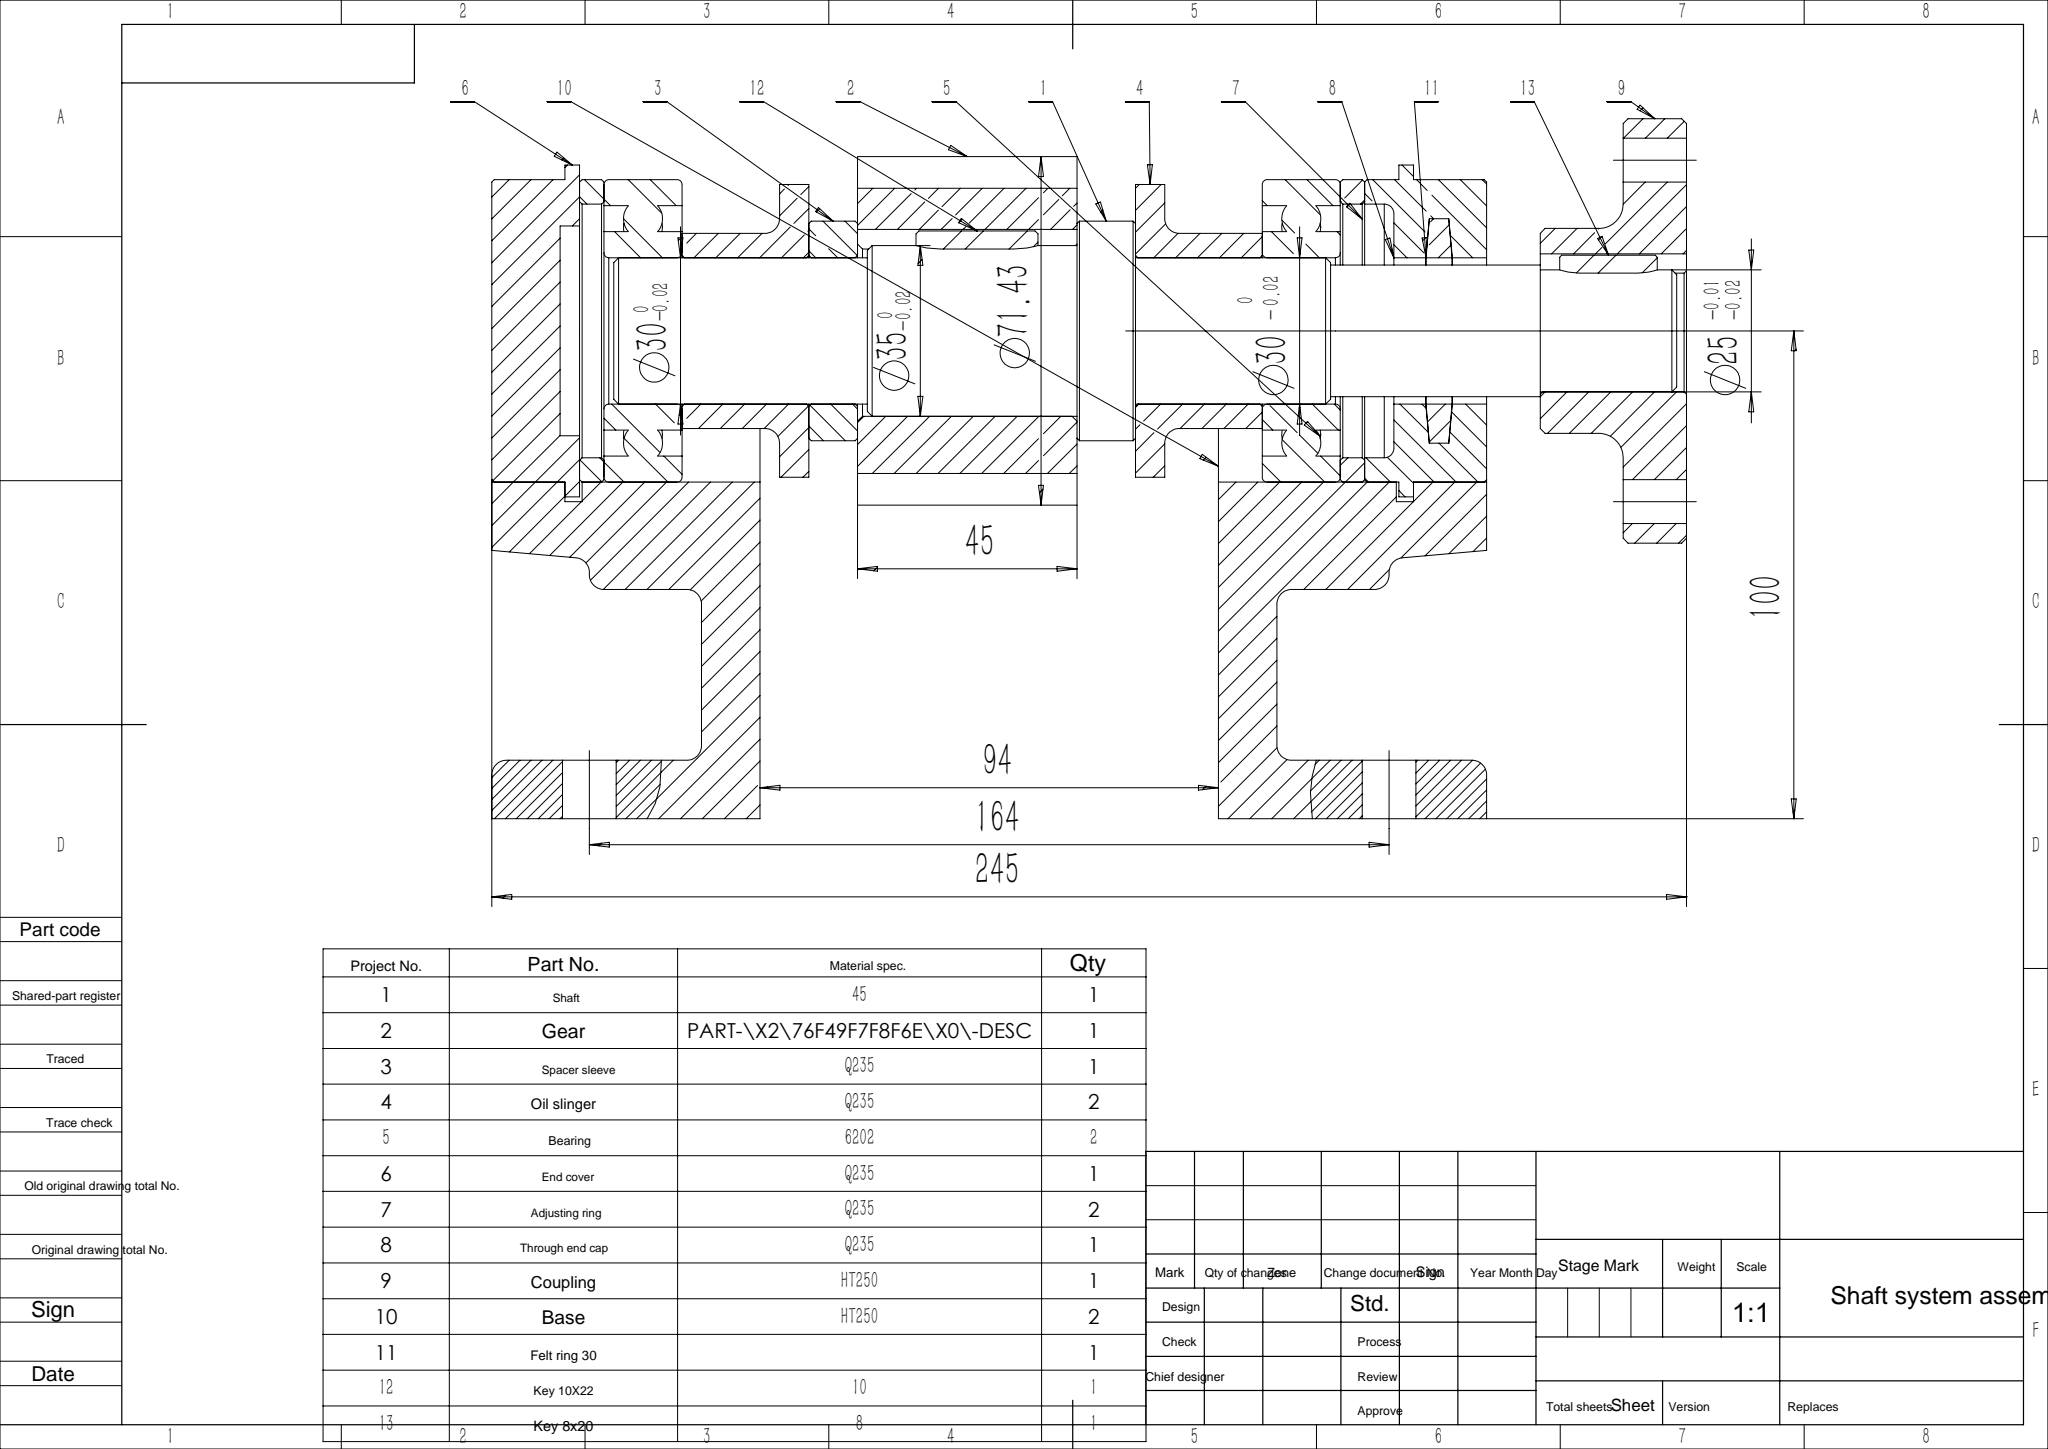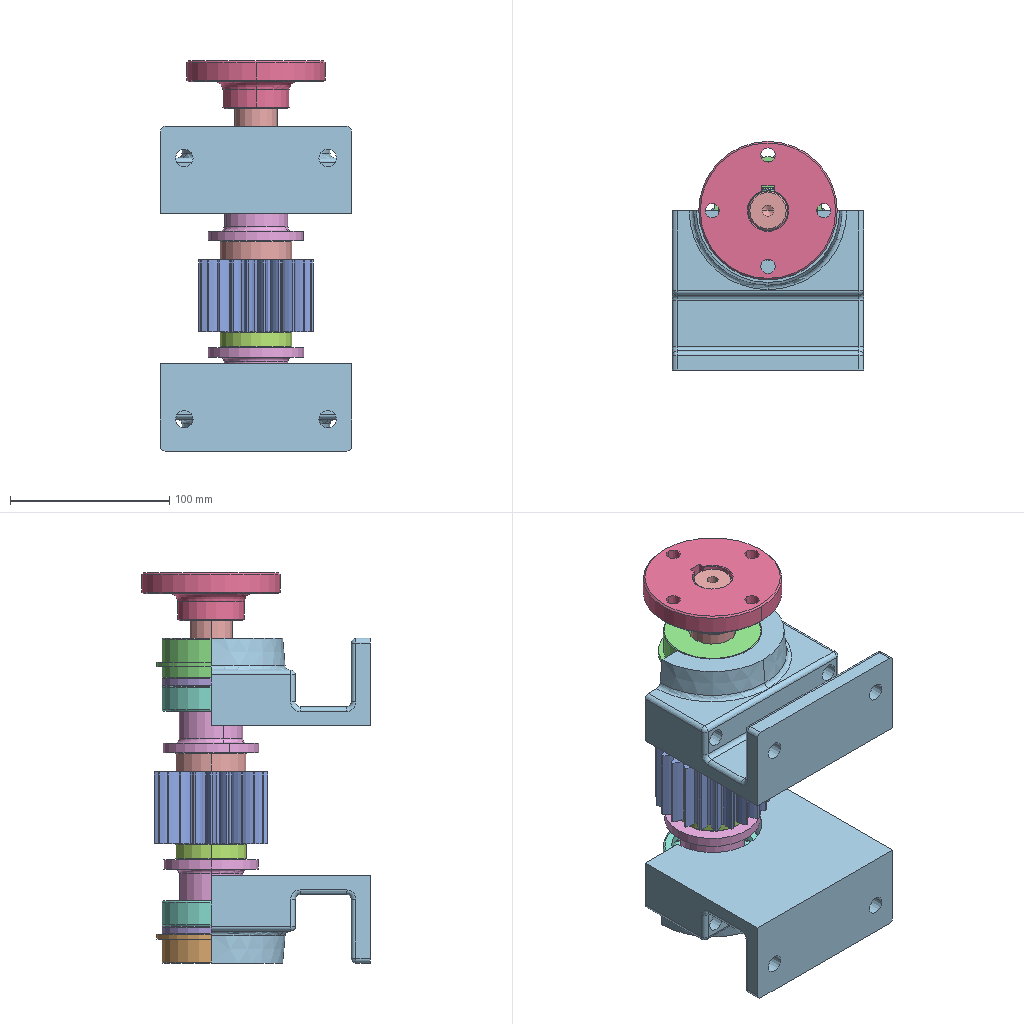Assembly | SolidWorks | 15 different items | 18 placed | box 120 x 144 x 245 mm
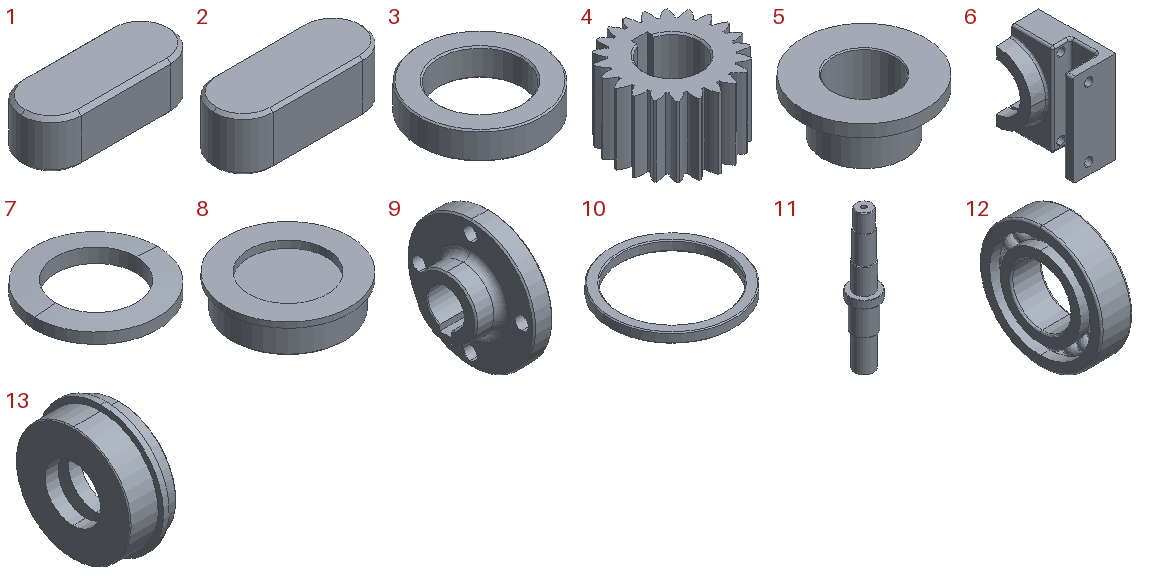Parts list (item | name | quantity | size | volume | features):
1 | - | x1 | 25 x 10 x 8 mm | 1807 mm3 | features Boss 2, Chamfer 1, Extrusion 1
2 | - | x1 | 20 x 8 x 7 mm | 1016 mm3 | features Boss 2, Chamfer 1, Extrusion 1
3 | - | x1 | 45 x 45 x 10 mm | 8777 mm3 | features Chamfer 1, Extrusion 1
4 | - | x1 | 71.989 x 71.433 x 45 mm | 107206 mm3 | features Chamfer 1, ICE 1, MBimport 1
5 | - | x2 | 60 x 60 x 26 mm | 23946 mm3 | features Chamfer 1, Extrusion 1, Fillet 1, ICE 1
6 | - | x2 | 55 x 100 x 120 mm | 321105 mm3 | features ICE 5, Fillet 4, Draft 1, Extrusion 1
7 | - | x1 | 46 x 46 x 5.333 mm | 4412 mm3 | features MBimport 1
8 | - | x1 | 68 x 68 x 18 mm | 50348 mm3 | features MBimport 1
9 | - | x1 | 30 x 87 x 87 mm | 82347 mm3 | features Chamfer 3, ICE 2, Fillet 1, Revolution 1
10 | - | x2 | 62 x 62 x 5 mm | 4387 mm3 | features Chamfer 1, Extrusion 1
11 | - | x1 | 45 x 45 x 218 mm | 161225 mm3 | features ICE 7, Chamfer 3, 3DProfileFeature 1, Extrusion 1, HoleWzd 1
12 | - | x1 | 16 x 62 x 62 mm | 27256 mm3 | features Revolution 3, CirPattern 1, Fillet 1
13 | - | x1 | 25 x 68 x 68 mm | 46745 mm3 | features MBimport 1
14 | deep groove ball bearings gb | x1 | - | - | -
15 | plain parallel keys | x1 | - | - | -
Mates (type | each side: item.copy, entity, surface, feature):
Parallel | 11.1 face plane Cut-Extrude1 | 4.1 face plane Cut-Extrude1
Concentric | 11.1 face cylinder Boss-Extrude2 | 4.1 face cylinder Gear.stp
Coincident | 11.1 face plane Boss-Extrude3 | 4.1 face plane Gear.stp
Coincident | 4.1 face plane Gear.stp | 3.1 face plane Boss-Extrude1
Concentric | 11.1 face cylinder Boss-Extrude1 | 3.1 face cylinder Boss-Extrude1
Coincident | 3.1 face plane Boss-Extrude1 | 5.1 face plane Boss-Extrude1
Concentric | 11.1 face cylinder Boss-Extrude1 | 5.1 face cylinder Boss-Extrude1
Coincident | 8.1 face plane Large Shaft End Cap.stp | 10.1 face plane Boss-Extrude1
Concentric | 11.1 face cylinder Boss-Extrude4 | 5.2 face cylinder Boss-Extrude1
Coincident | 11.1 face plane Boss-Extrude3 | 5.2 face plane Boss-Extrude1
Concentric | 11.1 face cylinder Boss-Extrude5 | 10.2 face cylinder Boss-Extrude1
Coincident | 10.2 face plane Boss-Extrude1 | 13.1 face plane Through End Cap (Large Shaft).stp
Concentric | 11.1 face cylinder Boss-Extrude5 | 13.1 face cylinder Through End Cap (Large Shaft).stp
Parallel | 11.1 face plane Cut-Extrude2 | 9.1 face plane Cut-Extrude2
Concentric | 11.1 face cylinder Boss-Extrude6 | 9.1 face cylinder Revolve1
Coincident | 11.1 face plane Boss-Extrude5 | 9.1 face plane Revolve1
Coincident | 8.1 face plane Large Shaft End Cap.stp | 6.1 face plane Cut-Extrude3
Concentric | 9.1 face cylinder Revolve1 | 6.2 face cylinder Cut-Extrude2
Coincident | 13.1 face plane Through End Cap (Large Shaft).stp | 6.2 face plane Cut-Extrude3
Concentric | 13.1 face cylinder Through End Cap (Large Shaft).stp | 7.1 face cylinder Felt Ring 30.stp